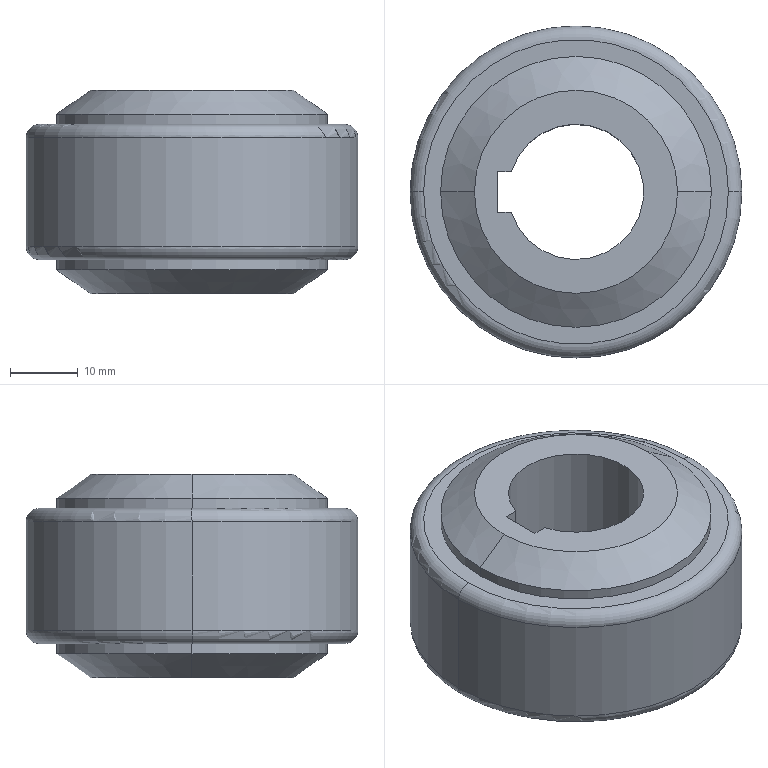Part | SolidWorks | features BaseBody 1 | 1 solid | 22 faces | box 49 x 49 x 30 mm | volume 38266 mm3 | cylinder 7 | plane 7 | torus 4 | cone 4 | commonest cylinder face diameters 40 x4 49 x2 20 x1
STEP:
#1=CARTESIAN_POINT('',(24.5,0.,18.));
#2=VERTEX_POINT('',#1);
#3=CARTESIAN_POINT('',(-24.5,0.,18.));
#4=VERTEX_POINT('',#3);
#5=CARTESIAN_POINT('',(0.,0.,18.));
#6=DIRECTION('',(0.,0.,1.));
#7=DIRECTION('',(-1.,0.,0.));
#8=AXIS2_PLACEMENT_3D('',#5,#6,#7);
#9=CIRCLE('',#8,24.5);
#10=EDGE_CURVE('',#2,#4,#9,.T.);
#11=ORIENTED_EDGE('',*,*,#10,.T.);
#12=CARTESIAN_POINT('',(-22.5,0.,20.));
#13=VERTEX_POINT('',#12);
#14=CARTESIAN_POINT('',(-22.5,0.,18.));
#15=DIRECTION('',(0.,1.,0.));
#16=DIRECTION('',(-1.,0.,0.));
#17=AXIS2_PLACEMENT_3D('',#14,#15,#16);
#18=CIRCLE('',#17,2.);
#19=EDGE_CURVE('',#4,#13,#18,.T.);
#20=ORIENTED_EDGE('',*,*,#19,.T.);
#21=CARTESIAN_POINT('',(22.5,0.,20.));
#22=VERTEX_POINT('',#21);
#23=CARTESIAN_POINT('',(0.,0.,20.));
#24=DIRECTION('',(0.,0.,-1.));
#25=DIRECTION('',(-1.,0.,0.));
#26=AXIS2_PLACEMENT_3D('',#23,#24,#25);
#27=CIRCLE('',#26,22.5);
#28=EDGE_CURVE('',#13,#22,#27,.T.);
#29=ORIENTED_EDGE('',*,*,#28,.T.);
#30=CARTESIAN_POINT('',(22.5,0.,18.));
#31=DIRECTION('',(0.,-1.,0.));
#32=DIRECTION('',(0.,0.,-1.));
#33=AXIS2_PLACEMENT_3D('',#30,#31,#32);
#34=CIRCLE('',#33,2.);
#35=EDGE_CURVE('',#2,#22,#34,.T.);
#36=ORIENTED_EDGE('',*,*,#35,.F.);
#37=EDGE_LOOP('',(#11,#20,#29,#36));
#38=FACE_OUTER_BOUND('',#37,.T.);
#39=CARTESIAN_POINT('',(0.,0.,18.));
#40=DIRECTION('',(0.,0.,1.));
#41=DIRECTION('',(1.,0.,0.));
#42=AXIS2_PLACEMENT_3D('',#39,#40,#41);
#43=TOROIDAL_SURFACE('',#42,22.5,2.);
#44=ADVANCED_FACE('',(#38),#43,.T.);
#45=ORIENTED_EDGE('',*,*,#10,.F.);
#46=CARTESIAN_POINT('',(24.5,0.,2.));
#47=VERTEX_POINT('',#46);
#48=CARTESIAN_POINT('',(24.5,0.,0.));
#49=DIRECTION('',(0.,0.,-1.));
#50=VECTOR('',#49,1000.);
#51=LINE('',#48,#50);
#52=EDGE_CURVE('',#2,#47,#51,.T.);
#53=ORIENTED_EDGE('',*,*,#52,.T.);
#54=CARTESIAN_POINT('',(-24.5,0.,2.));
#55=VERTEX_POINT('',#54);
#56=CARTESIAN_POINT('',(0.,0.,2.));
#57=DIRECTION('',(0.,0.,-1.));
#58=DIRECTION('',(-1.,0.,0.));
#59=AXIS2_PLACEMENT_3D('',#56,#57,#58);
#60=CIRCLE('',#59,24.5);
#61=EDGE_CURVE('',#55,#47,#60,.T.);
#62=ORIENTED_EDGE('',*,*,#61,.F.);
#63=CARTESIAN_POINT('',(-24.5,0.,0.));
#64=DIRECTION('',(0.,0.,-1.));
#65=VECTOR('',#64,1000.);
#66=LINE('',#63,#65);
#67=EDGE_CURVE('',#4,#55,#66,.T.);
#68=ORIENTED_EDGE('',*,*,#67,.F.);
#69=EDGE_LOOP('',(#45,#53,#62,#68));
#70=FACE_OUTER_BOUND('',#69,.T.);
#71=CARTESIAN_POINT('',(0.,0.,0.));
#72=DIRECTION('',(0.,0.,-1.));
#73=DIRECTION('',(-1.,0.,0.));
#74=AXIS2_PLACEMENT_3D('',#71,#72,#73);
#75=CYLINDRICAL_SURFACE('',#74,24.5);
#76=ADVANCED_FACE('',(#70),#75,.T.);
#77=ORIENTED_EDGE('',*,*,#61,.T.);
#78=CARTESIAN_POINT('',(22.5,0.,0.));
#79=VERTEX_POINT('',#78);
#80=CARTESIAN_POINT('',(22.5,0.,2.));
#81=DIRECTION('',(0.,1.,0.));
#82=DIRECTION('',(-1.,0.,0.));
#83=AXIS2_PLACEMENT_3D('',#80,#81,#82);
#84=CIRCLE('',#83,2.);
#85=EDGE_CURVE('',#47,#79,#84,.T.);
#86=ORIENTED_EDGE('',*,*,#85,.T.);
#87=CARTESIAN_POINT('',(-22.5,0.,0.));
#88=VERTEX_POINT('',#87);
#89=CARTESIAN_POINT('',(0.,0.,0.));
#90=DIRECTION('',(0.,0.,1.));
#91=DIRECTION('',(-1.,0.,0.));
#92=AXIS2_PLACEMENT_3D('',#89,#90,#91);
#93=CIRCLE('',#92,22.5);
#94=EDGE_CURVE('',#79,#88,#93,.T.);
#95=ORIENTED_EDGE('',*,*,#94,.T.);
#96=CARTESIAN_POINT('',(-22.5,0.,2.));
#97=DIRECTION('',(0.,-1.,0.));
#98=DIRECTION('',(0.,0.,-1.));
#99=AXIS2_PLACEMENT_3D('',#96,#97,#98);
#100=CIRCLE('',#99,2.);
#101=EDGE_CURVE('',#55,#88,#100,.T.);
#102=ORIENTED_EDGE('',*,*,#101,.F.);
#103=EDGE_LOOP('',(#77,#86,#95,#102));
#104=FACE_OUTER_BOUND('',#103,.T.);
#105=CARTESIAN_POINT('',(0.,0.,2.));
#106=DIRECTION('',(0.,0.,-1.));
#107=DIRECTION('',(-1.,0.,0.));
#108=AXIS2_PLACEMENT_3D('',#105,#106,#107);
#109=TOROIDAL_SURFACE('',#108,22.5,2.);
#110=ADVANCED_FACE('',(#104),#109,.T.);
#111=CARTESIAN_POINT('',(15.,0.,-5.));
#112=VERTEX_POINT('',#111);
#113=CARTESIAN_POINT('',(-15.,0.,-5.));
#114=VERTEX_POINT('',#113);
#115=CARTESIAN_POINT('',(0.,0.,-5.));
#116=DIRECTION('',(0.,0.,1.));
#117=DIRECTION('',(1.,0.,0.));
#118=AXIS2_PLACEMENT_3D('',#115,#116,#117);
#119=CIRCLE('',#118,15.);
#120=EDGE_CURVE('',#112,#114,#119,.T.);
#121=ORIENTED_EDGE('',*,*,#120,.T.);
#122=CARTESIAN_POINT('',(-20.,0.,-1.5));
#123=VERTEX_POINT('',#122);
#124=CARTESIAN_POINT('',(-17.5,0.,-3.25));
#125=DIRECTION('',(-0.8192,0.,0.5735));
#126=VECTOR('',#125,1000.);
#127=LINE('',#124,#126);
#128=EDGE_CURVE('',#114,#123,#127,.T.);
#129=ORIENTED_EDGE('',*,*,#128,.T.);
#130=CARTESIAN_POINT('',(20.,0.,-1.5));
#131=VERTEX_POINT('',#130);
#132=CARTESIAN_POINT('',(0.,0.,-1.5));
#133=DIRECTION('',(0.,0.,-1.));
#134=DIRECTION('',(1.,0.,0.));
#135=AXIS2_PLACEMENT_3D('',#132,#133,#134);
#136=CIRCLE('',#135,20.);
#137=EDGE_CURVE('',#123,#131,#136,.T.);
#138=ORIENTED_EDGE('',*,*,#137,.T.);
#139=CARTESIAN_POINT('',(17.5,0.,-3.25));
#140=DIRECTION('',(0.8192,0.,0.5735));
#141=VECTOR('',#140,1000.);
#142=LINE('',#139,#141);
#143=EDGE_CURVE('',#112,#131,#142,.T.);
#144=ORIENTED_EDGE('',*,*,#143,.F.);
#145=EDGE_LOOP('',(#121,#129,#138,#144));
#146=FACE_OUTER_BOUND('',#145,.T.);
#147=CARTESIAN_POINT('',(0.,0.,-3.25));
#148=DIRECTION('',(0.,0.,1.));
#149=DIRECTION('',(1.,0.,0.));
#150=AXIS2_PLACEMENT_3D('',#147,#148,#149);
#151=CONICAL_SURFACE('',#150,17.5,0.9601);
#152=ADVANCED_FACE('',(#146),#151,.T.);
#153=ORIENTED_EDGE('',*,*,#137,.F.);
#154=CARTESIAN_POINT('',(-20.,0.,0.));
#155=VERTEX_POINT('',#154);
#156=CARTESIAN_POINT('',(-20.,0.,0.));
#157=DIRECTION('',(0.,0.,1.));
#158=VECTOR('',#157,1000.);
#159=LINE('',#156,#158);
#160=EDGE_CURVE('',#123,#155,#159,.T.);
#161=ORIENTED_EDGE('',*,*,#160,.T.);
#162=CARTESIAN_POINT('',(20.,0.,0.));
#163=VERTEX_POINT('',#162);
#164=CARTESIAN_POINT('',(0.,0.,0.));
#165=DIRECTION('',(0.,0.,1.));
#166=DIRECTION('',(1.,0.,0.));
#167=AXIS2_PLACEMENT_3D('',#164,#165,#166);
#168=CIRCLE('',#167,20.);
#169=EDGE_CURVE('',#163,#155,#168,.T.);
#170=ORIENTED_EDGE('',*,*,#169,.F.);
#171=CARTESIAN_POINT('',(20.,0.,0.));
#172=DIRECTION('',(0.,0.,1.));
#173=VECTOR('',#172,1000.);
#174=LINE('',#171,#173);
#175=EDGE_CURVE('',#131,#163,#174,.T.);
#176=ORIENTED_EDGE('',*,*,#175,.F.);
#177=EDGE_LOOP('',(#153,#161,#170,#176));
#178=FACE_OUTER_BOUND('',#177,.T.);
#179=CARTESIAN_POINT('',(0.,0.,0.));
#180=DIRECTION('',(0.,0.,1.));
#181=DIRECTION('',(1.,0.,0.));
#182=AXIS2_PLACEMENT_3D('',#179,#180,#181);
#183=CYLINDRICAL_SURFACE('',#182,20.);
#184=ADVANCED_FACE('',(#178),#183,.T.);
#185=CARTESIAN_POINT('',(-15.,0.,25.));
#186=VERTEX_POINT('',#185);
#187=CARTESIAN_POINT('',(15.,0.,25.));
#188=VERTEX_POINT('',#187);
#189=CARTESIAN_POINT('',(0.,0.,25.));
#190=DIRECTION('',(0.,0.,-1.));
#191=DIRECTION('',(-1.,0.,0.));
#192=AXIS2_PLACEMENT_3D('',#189,#190,#191);
#193=CIRCLE('',#192,15.);
#194=EDGE_CURVE('',#186,#188,#193,.T.);
#195=ORIENTED_EDGE('',*,*,#194,.T.);
#196=CARTESIAN_POINT('',(20.,0.,21.5));
#197=VERTEX_POINT('',#196);
#198=CARTESIAN_POINT('',(17.5,0.,23.25));
#199=DIRECTION('',(0.8192,0.,-0.5735));
#200=VECTOR('',#199,1000.);
#201=LINE('',#198,#200);
#202=EDGE_CURVE('',#188,#197,#201,.T.);
#203=ORIENTED_EDGE('',*,*,#202,.T.);
#204=CARTESIAN_POINT('',(-20.,0.,21.5));
#205=VERTEX_POINT('',#204);
#206=CARTESIAN_POINT('',(0.,0.,21.5));
#207=DIRECTION('',(0.,0.,1.));
#208=DIRECTION('',(-1.,0.,0.));
#209=AXIS2_PLACEMENT_3D('',#206,#207,#208);
#210=CIRCLE('',#209,20.);
#211=EDGE_CURVE('',#197,#205,#210,.T.);
#212=ORIENTED_EDGE('',*,*,#211,.T.);
#213=CARTESIAN_POINT('',(-17.5,0.,23.25));
#214=DIRECTION('',(-0.8192,0.,-0.5735));
#215=VECTOR('',#214,1000.);
#216=LINE('',#213,#215);
#217=EDGE_CURVE('',#186,#205,#216,.T.);
#218=ORIENTED_EDGE('',*,*,#217,.F.);
#219=EDGE_LOOP('',(#195,#203,#212,#218));
#220=FACE_OUTER_BOUND('',#219,.T.);
#221=CARTESIAN_POINT('',(0.,0.,23.25));
#222=DIRECTION('',(0.,0.,-1.));
#223=DIRECTION('',(-1.,0.,0.));
#224=AXIS2_PLACEMENT_3D('',#221,#222,#223);
#225=CONICAL_SURFACE('',#224,17.5,0.9601);
#226=ADVANCED_FACE('',(#220),#225,.T.);
#227=ORIENTED_EDGE('',*,*,#211,.F.);
#228=CARTESIAN_POINT('',(20.,0.,20.));
#229=VERTEX_POINT('',#228);
#230=CARTESIAN_POINT('',(20.,0.,20.));
#231=DIRECTION('',(0.,0.,-1.));
#232=VECTOR('',#231,1000.);
#233=LINE('',#230,#232);
#234=EDGE_CURVE('',#197,#229,#233,.T.);
#235=ORIENTED_EDGE('',*,*,#234,.T.);
#236=CARTESIAN_POINT('',(-20.,0.,20.));
#237=VERTEX_POINT('',#236);
#238=CARTESIAN_POINT('',(0.,0.,20.));
#239=DIRECTION('',(0.,0.,-1.));
#240=DIRECTION('',(-1.,0.,0.));
#241=AXIS2_PLACEMENT_3D('',#238,#239,#240);
#242=CIRCLE('',#241,20.);
#243=EDGE_CURVE('',#237,#229,#242,.T.);
#244=ORIENTED_EDGE('',*,*,#243,.F.);
#245=CARTESIAN_POINT('',(-20.,0.,20.));
#246=DIRECTION('',(0.,0.,-1.));
#247=VECTOR('',#246,1000.);
#248=LINE('',#245,#247);
#249=EDGE_CURVE('',#205,#237,#248,.T.);
#250=ORIENTED_EDGE('',*,*,#249,.F.);
#251=EDGE_LOOP('',(#227,#235,#244,#250));
#252=FACE_OUTER_BOUND('',#251,.T.);
#253=CARTESIAN_POINT('',(0.,0.,20.));
#254=DIRECTION('',(0.,0.,-1.));
#255=DIRECTION('',(-1.,0.,0.));
#256=AXIS2_PLACEMENT_3D('',#253,#254,#255);
#257=CYLINDRICAL_SURFACE('',#256,20.);
#258=ADVANCED_FACE('',(#252),#257,.T.);
#259=CARTESIAN_POINT('',(-11.6,-3.,25.));
#260=VERTEX_POINT('',#259);
#261=CARTESIAN_POINT('',(-11.6,3.,25.));
#262=VERTEX_POINT('',#261);
#263=CARTESIAN_POINT('',(-11.6,1.5,25.));
#264=DIRECTION('',(0.,1.,0.));
#265=VECTOR('',#264,1000.);
#266=LINE('',#263,#265);
#267=EDGE_CURVE('',#260,#262,#266,.T.);
#268=ORIENTED_EDGE('',*,*,#267,.F.);
#269=CARTESIAN_POINT('',(-11.6,-3.,-5.));
#270=VERTEX_POINT('',#269);
#271=CARTESIAN_POINT('',(-11.6,-3.,-5.));
#272=DIRECTION('',(0.,0.,1.));
#273=VECTOR('',#272,1000.);
#274=LINE('',#271,#273);
#275=EDGE_CURVE('',#270,#260,#274,.T.);
#276=ORIENTED_EDGE('',*,*,#275,.F.);
#277=CARTESIAN_POINT('',(-11.6,3.,-5.));
#278=VERTEX_POINT('',#277);
#279=CARTESIAN_POINT('',(-11.6,1.5,-5.));
#280=DIRECTION('',(0.,-1.,0.));
#281=VECTOR('',#280,1000.);
#282=LINE('',#279,#281);
#283=EDGE_CURVE('',#278,#270,#282,.T.);
#284=ORIENTED_EDGE('',*,*,#283,.F.);
#285=CARTESIAN_POINT('',(-11.6,3.,-5.));
#286=DIRECTION('',(0.,0.,1.));
#287=VECTOR('',#286,1000.);
#288=LINE('',#285,#287);
#289=EDGE_CURVE('',#278,#262,#288,.T.);
#290=ORIENTED_EDGE('',*,*,#289,.T.);
#291=EDGE_LOOP('',(#268,#276,#284,#290));
#292=FACE_OUTER_BOUND('',#291,.T.);
#293=CARTESIAN_POINT('',(-11.6,3.,-5.));
#294=DIRECTION('',(-1.,0.,0.));
#295=DIRECTION('',(0.,0.,1.));
#296=AXIS2_PLACEMENT_3D('',#293,#294,#295);
#297=PLANE('',#296);
#298=ADVANCED_FACE('',(#292),#297,.F.);
#299=CARTESIAN_POINT('',(-9.539,3.,25.));
#300=VERTEX_POINT('',#299);
#301=CARTESIAN_POINT('',(-4.77,3.,25.));
#302=DIRECTION('',(1.,0.,0.));
#303=VECTOR('',#302,1000.);
#304=LINE('',#301,#303);
#305=EDGE_CURVE('',#262,#300,#304,.T.);
#306=ORIENTED_EDGE('',*,*,#305,.F.);
#307=ORIENTED_EDGE('',*,*,#289,.F.);
#308=CARTESIAN_POINT('',(-9.539,3.,-5.));
#309=VERTEX_POINT('',#308);
#310=CARTESIAN_POINT('',(-4.77,3.,-5.));
#311=DIRECTION('',(-1.,0.,0.));
#312=VECTOR('',#311,1000.);
#313=LINE('',#310,#312);
#314=EDGE_CURVE('',#309,#278,#313,.T.);
#315=ORIENTED_EDGE('',*,*,#314,.F.);
#316=CARTESIAN_POINT('',(-9.539,3.,-5.));
#317=DIRECTION('',(0.,0.,1.));
#318=VECTOR('',#317,1000.);
#319=LINE('',#316,#318);
#320=EDGE_CURVE('',#309,#300,#319,.T.);
#321=ORIENTED_EDGE('',*,*,#320,.T.);
#322=EDGE_LOOP('',(#306,#307,#315,#321));
#323=FACE_OUTER_BOUND('',#322,.T.);
#324=CARTESIAN_POINT('',(-9.539,3.,-5.));
#325=DIRECTION('',(0.,1.,0.));
#326=DIRECTION('',(1.,0.,0.));
#327=AXIS2_PLACEMENT_3D('',#324,#325,#326);
#328=PLANE('',#327);
#329=ADVANCED_FACE('',(#323),#328,.F.);
#330=CARTESIAN_POINT('',(-9.539,-3.,25.));
#331=VERTEX_POINT('',#330);
#332=CARTESIAN_POINT('',(0.,0.,25.));
#333=DIRECTION('',(0.,0.,-1.));
#334=DIRECTION('',(-1.,0.,0.));
#335=AXIS2_PLACEMENT_3D('',#332,#333,#334);
#336=CIRCLE('',#335,10.);
#337=EDGE_CURVE('',#300,#331,#336,.T.);
#338=ORIENTED_EDGE('',*,*,#337,.F.);
#339=ORIENTED_EDGE('',*,*,#320,.F.);
#340=CARTESIAN_POINT('',(-9.539,-3.,-5.));
#341=VERTEX_POINT('',#340);
#342=CARTESIAN_POINT('',(0.,0.,-5.));
#343=DIRECTION('',(0.,0.,1.));
#344=DIRECTION('',(-1.,0.,0.));
#345=AXIS2_PLACEMENT_3D('',#342,#343,#344);
#346=CIRCLE('',#345,10.);
#347=EDGE_CURVE('',#341,#309,#346,.T.);
#348=ORIENTED_EDGE('',*,*,#347,.F.);
#349=CARTESIAN_POINT('',(-9.539,-3.,-5.));
#350=DIRECTION('',(0.,0.,1.));
#351=VECTOR('',#350,1000.);
#352=LINE('',#349,#351);
#353=EDGE_CURVE('',#341,#331,#352,.T.);
#354=ORIENTED_EDGE('',*,*,#353,.T.);
#355=EDGE_LOOP('',(#338,#339,#348,#354));
#356=FACE_OUTER_BOUND('',#355,.T.);
#357=CARTESIAN_POINT('',(0.,0.,-5.));
#358=DIRECTION('',(0.,0.,-1.));
#359=DIRECTION('',(-1.,0.,0.));
#360=AXIS2_PLACEMENT_3D('',#357,#358,#359);
#361=CYLINDRICAL_SURFACE('',#360,10.);
#362=ADVANCED_FACE('',(#356),#361,.F.);
#363=CARTESIAN_POINT('',(-5.8,-3.,25.));
#364=DIRECTION('',(-1.,0.,0.));
#365=VECTOR('',#364,1000.);
#366=LINE('',#363,#365);
#367=EDGE_CURVE('',#331,#260,#366,.T.);
#368=ORIENTED_EDGE('',*,*,#367,.F.);
#369=ORIENTED_EDGE('',*,*,#353,.F.);
#370=CARTESIAN_POINT('',(-5.8,-3.,-5.));
#371=DIRECTION('',(1.,0.,0.));
#372=VECTOR('',#371,1000.);
#373=LINE('',#370,#372);
#374=EDGE_CURVE('',#270,#341,#373,.T.);
#375=ORIENTED_EDGE('',*,*,#374,.F.);
#376=ORIENTED_EDGE('',*,*,#275,.T.);
#377=EDGE_LOOP('',(#368,#369,#375,#376));
#378=FACE_OUTER_BOUND('',#377,.T.);
#379=CARTESIAN_POINT('',(-11.6,-3.,-5.));
#380=DIRECTION('',(0.,-1.,0.));
#381=DIRECTION('',(-1.,0.,0.));
#382=AXIS2_PLACEMENT_3D('',#379,#380,#381);
#383=PLANE('',#382);
#384=ADVANCED_FACE('',(#378),#383,.F.);
#385=ORIENTED_EDGE('',*,*,#243,.T.);
#386=CARTESIAN_POINT('',(0.,0.,20.));
#387=DIRECTION('',(0.,0.,-1.));
#388=DIRECTION('',(-1.,0.,0.));
#389=AXIS2_PLACEMENT_3D('',#386,#387,#388);
#390=CIRCLE('',#389,20.);
#391=EDGE_CURVE('',#229,#237,#390,.T.);
#392=ORIENTED_EDGE('',*,*,#391,.T.);
#393=EDGE_LOOP('',(#385,#392));
#394=FACE_BOUND('',#393,.T.);
#395=CARTESIAN_POINT('',(0.,0.,20.));
#396=DIRECTION('',(0.,0.,-1.));
#397=DIRECTION('',(-1.,0.,0.));
#398=AXIS2_PLACEMENT_3D('',#395,#396,#397);
#399=CIRCLE('',#398,22.5);
#400=EDGE_CURVE('',#22,#13,#399,.T.);
#401=ORIENTED_EDGE('',*,*,#400,.F.);
#402=ORIENTED_EDGE('',*,*,#28,.F.);
#403=EDGE_LOOP('',(#401,#402));
#404=FACE_OUTER_BOUND('',#403,.T.);
#405=CARTESIAN_POINT('',(0.,0.,20.));
#406=DIRECTION('',(0.,0.,1.));
#407=DIRECTION('',(1.,0.,0.));
#408=AXIS2_PLACEMENT_3D('',#405,#406,#407);
#409=PLANE('',#408);
#410=ADVANCED_FACE('',(#394,#404),#409,.T.);
#411=ORIENTED_EDGE('',*,*,#169,.T.);
#412=CARTESIAN_POINT('',(0.,0.,0.));
#413=DIRECTION('',(0.,0.,1.));
#414=DIRECTION('',(1.,0.,0.));
#415=AXIS2_PLACEMENT_3D('',#412,#413,#414);
#416=CIRCLE('',#415,20.);
#417=EDGE_CURVE('',#155,#163,#416,.T.);
#418=ORIENTED_EDGE('',*,*,#417,.T.);
#419=EDGE_LOOP('',(#411,#418));
#420=FACE_BOUND('',#419,.T.);
#421=CARTESIAN_POINT('',(0.,0.,0.));
#422=DIRECTION('',(0.,0.,1.));
#423=DIRECTION('',(-1.,0.,0.));
#424=AXIS2_PLACEMENT_3D('',#421,#422,#423);
#425=CIRCLE('',#424,22.5);
#426=EDGE_CURVE('',#88,#79,#425,.T.);
#427=ORIENTED_EDGE('',*,*,#426,.F.);
#428=ORIENTED_EDGE('',*,*,#94,.F.);
#429=EDGE_LOOP('',(#427,#428));
#430=FACE_OUTER_BOUND('',#429,.T.);
#431=CARTESIAN_POINT('',(0.,0.,0.));
#432=DIRECTION('',(0.,0.,1.));
#433=DIRECTION('',(1.,0.,0.));
#434=AXIS2_PLACEMENT_3D('',#431,#432,#433);
#435=PLANE('',#434);
#436=ADVANCED_FACE('',(#420,#430),#435,.F.);
#437=ORIENTED_EDGE('',*,*,#347,.T.);
#438=ORIENTED_EDGE('',*,*,#314,.T.);
#439=ORIENTED_EDGE('',*,*,#283,.T.);
#440=ORIENTED_EDGE('',*,*,#374,.T.);
#441=EDGE_LOOP('',(#437,#438,#439,#440));
#442=FACE_BOUND('',#441,.T.);
#443=ORIENTED_EDGE('',*,*,#120,.F.);
#444=CARTESIAN_POINT('',(0.,0.,-5.));
#445=DIRECTION('',(0.,0.,1.));
#446=DIRECTION('',(1.,0.,0.));
#447=AXIS2_PLACEMENT_3D('',#444,#445,#446);
#448=CIRCLE('',#447,15.);
#449=EDGE_CURVE('',#114,#112,#448,.T.);
#450=ORIENTED_EDGE('',*,*,#449,.F.);
#451=EDGE_LOOP('',(#443,#450));
#452=FACE_OUTER_BOUND('',#451,.T.);
#453=CARTESIAN_POINT('',(0.,0.,-5.));
#454=DIRECTION('',(0.,0.,1.));
#455=DIRECTION('',(1.,0.,0.));
#456=AXIS2_PLACEMENT_3D('',#453,#454,#455);
#457=PLANE('',#456);
#458=ADVANCED_FACE('',(#442,#452),#457,.F.);
#459=ORIENTED_EDGE('',*,*,#337,.T.);
#460=ORIENTED_EDGE('',*,*,#367,.T.);
#461=ORIENTED_EDGE('',*,*,#267,.T.);
#462=ORIENTED_EDGE('',*,*,#305,.T.);
#463=EDGE_LOOP('',(#459,#460,#461,#462));
#464=FACE_BOUND('',#463,.T.);
#465=ORIENTED_EDGE('',*,*,#194,.F.);
#466=CARTESIAN_POINT('',(0.,0.,25.));
#467=DIRECTION('',(0.,0.,-1.));
#468=DIRECTION('',(-1.,0.,0.));
#469=AXIS2_PLACEMENT_3D('',#466,#467,#468);
#470=CIRCLE('',#469,15.);
#471=EDGE_CURVE('',#188,#186,#470,.T.);
#472=ORIENTED_EDGE('',*,*,#471,.F.);
#473=EDGE_LOOP('',(#465,#472));
#474=FACE_OUTER_BOUND('',#473,.T.);
#475=CARTESIAN_POINT('',(0.,0.,25.));
#476=DIRECTION('',(0.,0.,1.));
#477=DIRECTION('',(1.,0.,0.));
#478=AXIS2_PLACEMENT_3D('',#475,#476,#477);
#479=PLANE('',#478);
#480=ADVANCED_FACE('',(#464,#474),#479,.T.);
#481=ORIENTED_EDGE('',*,*,#234,.F.);
#482=CARTESIAN_POINT('',(0.,0.,21.5));
#483=DIRECTION('',(0.,0.,1.));
#484=DIRECTION('',(-1.,0.,0.));
#485=AXIS2_PLACEMENT_3D('',#482,#483,#484);
#486=CIRCLE('',#485,20.);
#487=EDGE_CURVE('',#205,#197,#486,.T.);
#488=ORIENTED_EDGE('',*,*,#487,.F.);
#489=ORIENTED_EDGE('',*,*,#249,.T.);
#490=ORIENTED_EDGE('',*,*,#391,.F.);
#491=EDGE_LOOP('',(#481,#488,#489,#490));
#492=FACE_OUTER_BOUND('',#491,.T.);
#493=CARTESIAN_POINT('',(0.,0.,20.));
#494=DIRECTION('',(0.,0.,-1.));
#495=DIRECTION('',(-1.,0.,0.));
#496=AXIS2_PLACEMENT_3D('',#493,#494,#495);
#497=CYLINDRICAL_SURFACE('',#496,20.);
#498=ADVANCED_FACE('',(#492),#497,.T.);
#499=ORIENTED_EDGE('',*,*,#202,.F.);
#500=ORIENTED_EDGE('',*,*,#471,.T.);
#501=ORIENTED_EDGE('',*,*,#217,.T.);
#502=ORIENTED_EDGE('',*,*,#487,.T.);
#503=EDGE_LOOP('',(#499,#500,#501,#502));
#504=FACE_OUTER_BOUND('',#503,.T.);
#505=CARTESIAN_POINT('',(0.,0.,23.25));
#506=DIRECTION('',(0.,0.,-1.));
#507=DIRECTION('',(-1.,0.,0.));
#508=AXIS2_PLACEMENT_3D('',#505,#506,#507);
#509=CONICAL_SURFACE('',#508,17.5,0.9601);
#510=ADVANCED_FACE('',(#504),#509,.T.);
#511=ORIENTED_EDGE('',*,*,#160,.F.);
#512=CARTESIAN_POINT('',(0.,0.,-1.5));
#513=DIRECTION('',(0.,0.,-1.));
#514=DIRECTION('',(1.,0.,0.));
#515=AXIS2_PLACEMENT_3D('',#512,#513,#514);
#516=CIRCLE('',#515,20.);
#517=EDGE_CURVE('',#131,#123,#516,.T.);
#518=ORIENTED_EDGE('',*,*,#517,.F.);
#519=ORIENTED_EDGE('',*,*,#175,.T.);
#520=ORIENTED_EDGE('',*,*,#417,.F.);
#521=EDGE_LOOP('',(#511,#518,#519,#520));
#522=FACE_OUTER_BOUND('',#521,.T.);
#523=CARTESIAN_POINT('',(0.,0.,0.));
#524=DIRECTION('',(0.,0.,1.));
#525=DIRECTION('',(1.,0.,0.));
#526=AXIS2_PLACEMENT_3D('',#523,#524,#525);
#527=CYLINDRICAL_SURFACE('',#526,20.);
#528=ADVANCED_FACE('',(#522),#527,.T.);
#529=ORIENTED_EDGE('',*,*,#128,.F.);
#530=ORIENTED_EDGE('',*,*,#449,.T.);
#531=ORIENTED_EDGE('',*,*,#143,.T.);
#532=ORIENTED_EDGE('',*,*,#517,.T.);
#533=EDGE_LOOP('',(#529,#530,#531,#532));
#534=FACE_OUTER_BOUND('',#533,.T.);
#535=CARTESIAN_POINT('',(0.,0.,-3.25));
#536=DIRECTION('',(0.,0.,1.));
#537=DIRECTION('',(1.,0.,0.));
#538=AXIS2_PLACEMENT_3D('',#535,#536,#537);
#539=CONICAL_SURFACE('',#538,17.5,0.9601);
#540=ADVANCED_FACE('',(#534),#539,.T.);
#541=ORIENTED_EDGE('',*,*,#85,.F.);
#542=CARTESIAN_POINT('',(0.,0.,2.));
#543=DIRECTION('',(0.,0.,-1.));
#544=DIRECTION('',(-1.,0.,0.));
#545=AXIS2_PLACEMENT_3D('',#542,#543,#544);
#546=CIRCLE('',#545,24.5);
#547=EDGE_CURVE('',#47,#55,#546,.T.);
#548=ORIENTED_EDGE('',*,*,#547,.T.);
#549=ORIENTED_EDGE('',*,*,#101,.T.);
#550=ORIENTED_EDGE('',*,*,#426,.T.);
#551=EDGE_LOOP('',(#541,#548,#549,#550));
#552=FACE_OUTER_BOUND('',#551,.T.);
#553=CARTESIAN_POINT('',(0.,0.,2.));
#554=DIRECTION('',(0.,0.,-1.));
#555=DIRECTION('',(-1.,0.,0.));
#556=AXIS2_PLACEMENT_3D('',#553,#554,#555);
#557=TOROIDAL_SURFACE('',#556,22.5,2.);
#558=ADVANCED_FACE('',(#552),#557,.T.);
#559=ORIENTED_EDGE('',*,*,#52,.F.);
#560=CARTESIAN_POINT('',(0.,0.,18.));
#561=DIRECTION('',(0.,0.,1.));
#562=DIRECTION('',(-1.,0.,0.));
#563=AXIS2_PLACEMENT_3D('',#560,#561,#562);
#564=CIRCLE('',#563,24.5);
#565=EDGE_CURVE('',#4,#2,#564,.T.);
#566=ORIENTED_EDGE('',*,*,#565,.F.);
#567=ORIENTED_EDGE('',*,*,#67,.T.);
#568=ORIENTED_EDGE('',*,*,#547,.F.);
#569=EDGE_LOOP('',(#559,#566,#567,#568));
#570=FACE_OUTER_BOUND('',#569,.T.);
#571=CARTESIAN_POINT('',(0.,0.,0.));
#572=DIRECTION('',(0.,0.,-1.));
#573=DIRECTION('',(-1.,0.,0.));
#574=AXIS2_PLACEMENT_3D('',#571,#572,#573);
#575=CYLINDRICAL_SURFACE('',#574,24.5);
#576=ADVANCED_FACE('',(#570),#575,.T.);
#577=ORIENTED_EDGE('',*,*,#19,.F.);
#578=ORIENTED_EDGE('',*,*,#565,.T.);
#579=ORIENTED_EDGE('',*,*,#35,.T.);
#580=ORIENTED_EDGE('',*,*,#400,.T.);
#581=EDGE_LOOP('',(#577,#578,#579,#580));
#582=FACE_OUTER_BOUND('',#581,.T.);
#583=CARTESIAN_POINT('',(0.,0.,18.));
#584=DIRECTION('',(0.,0.,1.));
#585=DIRECTION('',(1.,0.,0.));
#586=AXIS2_PLACEMENT_3D('',#583,#584,#585);
#587=TOROIDAL_SURFACE('',#586,22.5,2.);
#588=ADVANCED_FACE('',(#582),#587,.T.);
#589=CLOSED_SHELL('',(#44,#76,#110,#152,#184,#226,#258,#298,#329,#362,#384,#410,#436,#458,#480,#498,#510,#528,#540,#558,#576,#588));
#590=MANIFOLD_SOLID_BREP('',#589);
#591=CARTESIAN_POINT('',(0.,0.,0.));
#592=DIRECTION('',(0.,0.,1.));
#593=DIRECTION('',(1.,0.,0.));
#594=AXIS2_PLACEMENT_3D('',#591,#592,#593);
#595=(LENGTH_UNIT()NAMED_UNIT(*)SI_UNIT(.MILLI.,.METRE.));
#596=UNCERTAINTY_MEASURE_WITH_UNIT(LENGTH_MEASURE(0.00001),#595,'','');
#597=(NAMED_UNIT(*)PLANE_ANGLE_UNIT()SI_UNIT($,.RADIAN.));
#598=(NAMED_UNIT(*)SI_UNIT($,.STERADIAN.)SOLID_ANGLE_UNIT());
#599=(GEOMETRIC_REPRESENTATION_CONTEXT(3)GLOBAL_UNCERTAINTY_ASSIGNED_CONTEXT((#596))GLOBAL_UNIT_ASSIGNED_CONTEXT((#595,#597,#598))REPRESENTATION_CONTEXT('',''));
#600=ADVANCED_BREP_SHAPE_REPRESENTATION('',(#590,#594),#599);